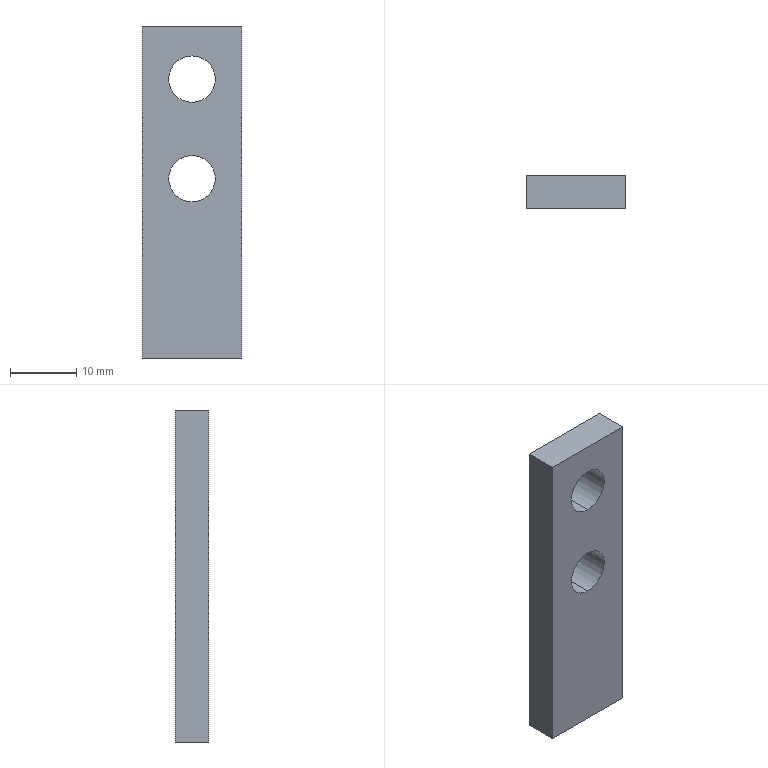Part | STEP file | 750038302 | 1 solid | 10 faces | box 15 x 5 x 50 mm | volume 3365 mm3 | plane 6 | cylinder 4 | commonest cylinder face diameters 7 x4
STEP:
#1=CARTESIAN_POINT('',(0.,2.5,45.5));
#2=VERTEX_POINT('',#1);
#3=CARTESIAN_POINT('',(0.,2.5,38.5));
#4=VERTEX_POINT('',#3);
#5=CARTESIAN_POINT('',(0.,2.5,42.));
#6=DIRECTION('',(0.,-1.,0.));
#7=DIRECTION('',(0.,0.,-1.));
#8=AXIS2_PLACEMENT_3D('',#5,#6,#7);
#9=CIRCLE('',#8,3.5);
#10=EDGE_CURVE('',#2,#4,#9,.T.);
#11=ORIENTED_EDGE('',*,*,#10,.F.);
#12=CARTESIAN_POINT('',(0.,-2.5,45.5));
#13=VERTEX_POINT('',#12);
#14=CARTESIAN_POINT('',(0.,54997.5,45.5));
#15=DIRECTION('',(0.,-1.,0.));
#16=VECTOR('',#15,1000.);
#17=LINE('',#14,#16);
#18=EDGE_CURVE('',#2,#13,#17,.T.);
#19=ORIENTED_EDGE('',*,*,#18,.T.);
#20=CARTESIAN_POINT('',(0.,-2.5,38.5));
#21=VERTEX_POINT('',#20);
#22=CARTESIAN_POINT('',(0.,-2.5,42.));
#23=DIRECTION('',(0.,-1.,0.));
#24=DIRECTION('',(0.,0.,-1.));
#25=AXIS2_PLACEMENT_3D('',#22,#23,#24);
#26=CIRCLE('',#25,3.5);
#27=EDGE_CURVE('',#13,#21,#26,.T.);
#28=ORIENTED_EDGE('',*,*,#27,.T.);
#29=CARTESIAN_POINT('',(0.,54997.5,38.5));
#30=DIRECTION('',(0.,-1.,0.));
#31=VECTOR('',#30,1000.);
#32=LINE('',#29,#31);
#33=EDGE_CURVE('',#4,#21,#32,.T.);
#34=ORIENTED_EDGE('',*,*,#33,.F.);
#35=EDGE_LOOP('',(#11,#19,#28,#34));
#36=FACE_OUTER_BOUND('',#35,.T.);
#37=CARTESIAN_POINT('',(0.,54997.5,42.));
#38=DIRECTION('',(0.,-1.,0.));
#39=DIRECTION('',(0.,0.,-1.));
#40=AXIS2_PLACEMENT_3D('',#37,#38,#39);
#41=CYLINDRICAL_SURFACE('',#40,3.5);
#42=ADVANCED_FACE('',(#36),#41,.F.);
#43=CARTESIAN_POINT('',(0.,2.5,30.5));
#44=VERTEX_POINT('',#43);
#45=CARTESIAN_POINT('',(0.,2.5,23.5));
#46=VERTEX_POINT('',#45);
#47=CARTESIAN_POINT('',(0.,2.5,27.));
#48=DIRECTION('',(0.,-1.,0.));
#49=DIRECTION('',(0.,0.,-1.));
#50=AXIS2_PLACEMENT_3D('',#47,#48,#49);
#51=CIRCLE('',#50,3.5);
#52=EDGE_CURVE('',#44,#46,#51,.T.);
#53=ORIENTED_EDGE('',*,*,#52,.F.);
#54=CARTESIAN_POINT('',(0.,-2.5,30.5));
#55=VERTEX_POINT('',#54);
#56=CARTESIAN_POINT('',(0.,54997.5,30.5));
#57=DIRECTION('',(0.,-1.,0.));
#58=VECTOR('',#57,1000.);
#59=LINE('',#56,#58);
#60=EDGE_CURVE('',#44,#55,#59,.T.);
#61=ORIENTED_EDGE('',*,*,#60,.T.);
#62=CARTESIAN_POINT('',(0.,-2.5,23.5));
#63=VERTEX_POINT('',#62);
#64=CARTESIAN_POINT('',(0.,-2.5,27.));
#65=DIRECTION('',(0.,-1.,0.));
#66=DIRECTION('',(0.,0.,-1.));
#67=AXIS2_PLACEMENT_3D('',#64,#65,#66);
#68=CIRCLE('',#67,3.5);
#69=EDGE_CURVE('',#55,#63,#68,.T.);
#70=ORIENTED_EDGE('',*,*,#69,.T.);
#71=CARTESIAN_POINT('',(0.,54997.5,23.5));
#72=DIRECTION('',(0.,-1.,0.));
#73=VECTOR('',#72,1000.);
#74=LINE('',#71,#73);
#75=EDGE_CURVE('',#46,#63,#74,.T.);
#76=ORIENTED_EDGE('',*,*,#75,.F.);
#77=EDGE_LOOP('',(#53,#61,#70,#76));
#78=FACE_OUTER_BOUND('',#77,.T.);
#79=CARTESIAN_POINT('',(0.,54997.5,27.));
#80=DIRECTION('',(0.,-1.,0.));
#81=DIRECTION('',(0.,0.,-1.));
#82=AXIS2_PLACEMENT_3D('',#79,#80,#81);
#83=CYLINDRICAL_SURFACE('',#82,3.5);
#84=ADVANCED_FACE('',(#78),#83,.F.);
#85=CARTESIAN_POINT('',(7.5,-2.5,50.));
#86=VERTEX_POINT('',#85);
#87=CARTESIAN_POINT('',(7.5,-2.5,0.));
#88=VERTEX_POINT('',#87);
#89=CARTESIAN_POINT('',(7.5,-2.5,50.));
#90=DIRECTION('',(0.,0.,-1.));
#91=VECTOR('',#90,1000.);
#92=LINE('',#89,#91);
#93=EDGE_CURVE('',#86,#88,#92,.T.);
#94=ORIENTED_EDGE('',*,*,#93,.F.);
#95=CARTESIAN_POINT('',(-7.5,-2.5,50.));
#96=VERTEX_POINT('',#95);
#97=CARTESIAN_POINT('',(-7.5,-2.5,50.));
#98=DIRECTION('',(1.,0.,0.));
#99=VECTOR('',#98,1000.);
#100=LINE('',#97,#99);
#101=EDGE_CURVE('',#96,#86,#100,.T.);
#102=ORIENTED_EDGE('',*,*,#101,.F.);
#103=CARTESIAN_POINT('',(-7.5,-2.5,0.));
#104=VERTEX_POINT('',#103);
#105=CARTESIAN_POINT('',(-7.5,-2.5,50.));
#106=DIRECTION('',(0.,0.,1.));
#107=VECTOR('',#106,1000.);
#108=LINE('',#105,#107);
#109=EDGE_CURVE('',#104,#96,#108,.T.);
#110=ORIENTED_EDGE('',*,*,#109,.F.);
#111=CARTESIAN_POINT('',(-7.5,-2.5,0.));
#112=DIRECTION('',(-1.,0.,0.));
#113=VECTOR('',#112,1000.);
#114=LINE('',#111,#113);
#115=EDGE_CURVE('',#88,#104,#114,.T.);
#116=ORIENTED_EDGE('',*,*,#115,.F.);
#117=EDGE_LOOP('',(#94,#102,#110,#116));
#118=FACE_OUTER_BOUND('',#117,.T.);
#119=CARTESIAN_POINT('',(0.,-2.5,42.));
#120=DIRECTION('',(0.,-1.,0.));
#121=DIRECTION('',(0.,0.,-1.));
#122=AXIS2_PLACEMENT_3D('',#119,#120,#121);
#123=CIRCLE('',#122,3.5);
#124=EDGE_CURVE('',#21,#13,#123,.T.);
#125=ORIENTED_EDGE('',*,*,#124,.F.);
#126=ORIENTED_EDGE('',*,*,#27,.F.);
#127=EDGE_LOOP('',(#125,#126));
#128=FACE_BOUND('',#127,.T.);
#129=CARTESIAN_POINT('',(0.,-2.5,27.));
#130=DIRECTION('',(0.,-1.,0.));
#131=DIRECTION('',(0.,0.,-1.));
#132=AXIS2_PLACEMENT_3D('',#129,#130,#131);
#133=CIRCLE('',#132,3.5);
#134=EDGE_CURVE('',#63,#55,#133,.T.);
#135=ORIENTED_EDGE('',*,*,#134,.F.);
#136=ORIENTED_EDGE('',*,*,#69,.F.);
#137=EDGE_LOOP('',(#135,#136));
#138=FACE_BOUND('',#137,.T.);
#139=CARTESIAN_POINT('',(-7.5,-2.5,50.));
#140=DIRECTION('',(0.,1.,0.));
#141=DIRECTION('',(0.,0.,1.));
#142=AXIS2_PLACEMENT_3D('',#139,#140,#141);
#143=PLANE('',#142);
#144=ADVANCED_FACE('',(#118,#128,#138),#143,.F.);
#145=CARTESIAN_POINT('',(-7.5,2.5,0.));
#146=VERTEX_POINT('',#145);
#147=CARTESIAN_POINT('',(-7.5,0.,0.));
#148=DIRECTION('',(0.,-1.,0.));
#149=VECTOR('',#148,1000.);
#150=LINE('',#147,#149);
#151=EDGE_CURVE('',#146,#104,#150,.T.);
#152=ORIENTED_EDGE('',*,*,#151,.F.);
#153=CARTESIAN_POINT('',(7.5,2.5,0.));
#154=VERTEX_POINT('',#153);
#155=CARTESIAN_POINT('',(0.,2.5,0.));
#156=DIRECTION('',(-1.,0.,0.));
#157=VECTOR('',#156,1000.);
#158=LINE('',#155,#157);
#159=EDGE_CURVE('',#154,#146,#158,.T.);
#160=ORIENTED_EDGE('',*,*,#159,.F.);
#161=CARTESIAN_POINT('',(7.5,0.,0.));
#162=DIRECTION('',(0.,1.,0.));
#163=VECTOR('',#162,1000.);
#164=LINE('',#161,#163);
#165=EDGE_CURVE('',#88,#154,#164,.T.);
#166=ORIENTED_EDGE('',*,*,#165,.F.);
#167=ORIENTED_EDGE('',*,*,#115,.T.);
#168=EDGE_LOOP('',(#152,#160,#166,#167));
#169=FACE_OUTER_BOUND('',#168,.T.);
#170=CARTESIAN_POINT('',(0.,0.,0.));
#171=DIRECTION('',(0.,0.,1.));
#172=DIRECTION('',(1.,0.,0.));
#173=AXIS2_PLACEMENT_3D('',#170,#171,#172);
#174=PLANE('',#173);
#175=ADVANCED_FACE('',(#169),#174,.F.);
#176=CARTESIAN_POINT('',(7.5,2.5,50.));
#177=VERTEX_POINT('',#176);
#178=CARTESIAN_POINT('',(7.5,2.5,50.));
#179=DIRECTION('',(0.,0.,-1.));
#180=VECTOR('',#179,1000.);
#181=LINE('',#178,#180);
#182=EDGE_CURVE('',#177,#154,#181,.T.);
#183=ORIENTED_EDGE('',*,*,#182,.F.);
#184=CARTESIAN_POINT('',(7.5,-2.5,50.));
#185=DIRECTION('',(0.,1.,0.));
#186=VECTOR('',#185,1000.);
#187=LINE('',#184,#186);
#188=EDGE_CURVE('',#86,#177,#187,.T.);
#189=ORIENTED_EDGE('',*,*,#188,.F.);
#190=ORIENTED_EDGE('',*,*,#93,.T.);
#191=ORIENTED_EDGE('',*,*,#165,.T.);
#192=EDGE_LOOP('',(#183,#189,#190,#191));
#193=FACE_OUTER_BOUND('',#192,.T.);
#194=CARTESIAN_POINT('',(7.5,-2.5,50.));
#195=DIRECTION('',(-1.,0.,0.));
#196=DIRECTION('',(0.,-1.,0.));
#197=AXIS2_PLACEMENT_3D('',#194,#195,#196);
#198=PLANE('',#197);
#199=ADVANCED_FACE('',(#193),#198,.F.);
#200=CARTESIAN_POINT('',(-7.5,2.5,50.));
#201=VERTEX_POINT('',#200);
#202=CARTESIAN_POINT('',(0.,2.5,50.));
#203=DIRECTION('',(-1.,0.,0.));
#204=VECTOR('',#203,1000.);
#205=LINE('',#202,#204);
#206=EDGE_CURVE('',#177,#201,#205,.T.);
#207=ORIENTED_EDGE('',*,*,#206,.T.);
#208=CARTESIAN_POINT('',(-7.5,0.,50.));
#209=DIRECTION('',(0.,-1.,0.));
#210=VECTOR('',#209,1000.);
#211=LINE('',#208,#210);
#212=EDGE_CURVE('',#201,#96,#211,.T.);
#213=ORIENTED_EDGE('',*,*,#212,.T.);
#214=ORIENTED_EDGE('',*,*,#101,.T.);
#215=ORIENTED_EDGE('',*,*,#188,.T.);
#216=EDGE_LOOP('',(#207,#213,#214,#215));
#217=FACE_OUTER_BOUND('',#216,.T.);
#218=CARTESIAN_POINT('',(0.,0.,50.));
#219=DIRECTION('',(0.,0.,1.));
#220=DIRECTION('',(1.,0.,0.));
#221=AXIS2_PLACEMENT_3D('',#218,#219,#220);
#222=PLANE('',#221);
#223=ADVANCED_FACE('',(#217),#222,.T.);
#224=ORIENTED_EDGE('',*,*,#109,.T.);
#225=ORIENTED_EDGE('',*,*,#212,.F.);
#226=CARTESIAN_POINT('',(-7.5,2.5,50.));
#227=DIRECTION('',(0.,0.,1.));
#228=VECTOR('',#227,1000.);
#229=LINE('',#226,#228);
#230=EDGE_CURVE('',#146,#201,#229,.T.);
#231=ORIENTED_EDGE('',*,*,#230,.F.);
#232=ORIENTED_EDGE('',*,*,#151,.T.);
#233=EDGE_LOOP('',(#224,#225,#231,#232));
#234=FACE_OUTER_BOUND('',#233,.T.);
#235=CARTESIAN_POINT('',(-7.5,2.5,50.));
#236=DIRECTION('',(1.,0.,0.));
#237=DIRECTION('',(0.,1.,0.));
#238=AXIS2_PLACEMENT_3D('',#235,#236,#237);
#239=PLANE('',#238);
#240=ADVANCED_FACE('',(#234),#239,.F.);
#241=ORIENTED_EDGE('',*,*,#18,.F.);
#242=CARTESIAN_POINT('',(0.,2.5,42.));
#243=DIRECTION('',(0.,-1.,0.));
#244=DIRECTION('',(0.,0.,-1.));
#245=AXIS2_PLACEMENT_3D('',#242,#243,#244);
#246=CIRCLE('',#245,3.5);
#247=EDGE_CURVE('',#4,#2,#246,.T.);
#248=ORIENTED_EDGE('',*,*,#247,.F.);
#249=ORIENTED_EDGE('',*,*,#33,.T.);
#250=ORIENTED_EDGE('',*,*,#124,.T.);
#251=EDGE_LOOP('',(#241,#248,#249,#250));
#252=FACE_OUTER_BOUND('',#251,.T.);
#253=CARTESIAN_POINT('',(0.,54997.5,42.));
#254=DIRECTION('',(0.,-1.,0.));
#255=DIRECTION('',(0.,0.,-1.));
#256=AXIS2_PLACEMENT_3D('',#253,#254,#255);
#257=CYLINDRICAL_SURFACE('',#256,3.5);
#258=ADVANCED_FACE('',(#252),#257,.F.);
#259=ORIENTED_EDGE('',*,*,#60,.F.);
#260=CARTESIAN_POINT('',(0.,2.5,27.));
#261=DIRECTION('',(0.,-1.,0.));
#262=DIRECTION('',(0.,0.,-1.));
#263=AXIS2_PLACEMENT_3D('',#260,#261,#262);
#264=CIRCLE('',#263,3.5);
#265=EDGE_CURVE('',#46,#44,#264,.T.);
#266=ORIENTED_EDGE('',*,*,#265,.F.);
#267=ORIENTED_EDGE('',*,*,#75,.T.);
#268=ORIENTED_EDGE('',*,*,#134,.T.);
#269=EDGE_LOOP('',(#259,#266,#267,#268));
#270=FACE_OUTER_BOUND('',#269,.T.);
#271=CARTESIAN_POINT('',(0.,54997.5,27.));
#272=DIRECTION('',(0.,-1.,0.));
#273=DIRECTION('',(0.,0.,-1.));
#274=AXIS2_PLACEMENT_3D('',#271,#272,#273);
#275=CYLINDRICAL_SURFACE('',#274,3.5);
#276=ADVANCED_FACE('',(#270),#275,.F.);
#277=ORIENTED_EDGE('',*,*,#230,.T.);
#278=ORIENTED_EDGE('',*,*,#206,.F.);
#279=ORIENTED_EDGE('',*,*,#182,.T.);
#280=ORIENTED_EDGE('',*,*,#159,.T.);
#281=EDGE_LOOP('',(#277,#278,#279,#280));
#282=FACE_OUTER_BOUND('',#281,.T.);
#283=ORIENTED_EDGE('',*,*,#247,.T.);
#284=ORIENTED_EDGE('',*,*,#10,.T.);
#285=EDGE_LOOP('',(#283,#284));
#286=FACE_BOUND('',#285,.T.);
#287=ORIENTED_EDGE('',*,*,#265,.T.);
#288=ORIENTED_EDGE('',*,*,#52,.T.);
#289=EDGE_LOOP('',(#287,#288));
#290=FACE_BOUND('',#289,.T.);
#291=CARTESIAN_POINT('',(7.5,2.5,50.));
#292=DIRECTION('',(0.,-1.,0.));
#293=DIRECTION('',(0.,0.,-1.));
#294=AXIS2_PLACEMENT_3D('',#291,#292,#293);
#295=PLANE('',#294);
#296=ADVANCED_FACE('',(#282,#286,#290),#295,.F.);
#297=CLOSED_SHELL('',(#42,#84,#144,#175,#199,#223,#240,#258,#276,#296));
#298=MANIFOLD_SOLID_BREP('',#297);
#299=CARTESIAN_POINT('',(0.,0.,0.));
#300=DIRECTION('',(0.,0.,1.));
#301=DIRECTION('',(1.,0.,0.));
#302=AXIS2_PLACEMENT_3D('',#299,#300,#301);
#303=(LENGTH_UNIT()NAMED_UNIT(*)SI_UNIT(.MILLI.,.METRE.));
#304=UNCERTAINTY_MEASURE_WITH_UNIT(LENGTH_MEASURE(0.00001),#303,'','');
#305=(NAMED_UNIT(*)PLANE_ANGLE_UNIT()SI_UNIT($,.RADIAN.));
#306=(NAMED_UNIT(*)SI_UNIT($,.STERADIAN.)SOLID_ANGLE_UNIT());
#307=(GEOMETRIC_REPRESENTATION_CONTEXT(3)GLOBAL_UNCERTAINTY_ASSIGNED_CONTEXT((#304))GLOBAL_UNIT_ASSIGNED_CONTEXT((#303,#305,#306))REPRESENTATION_CONTEXT('',''));
#308=ADVANCED_BREP_SHAPE_REPRESENTATION('',(#298,#302),#307);